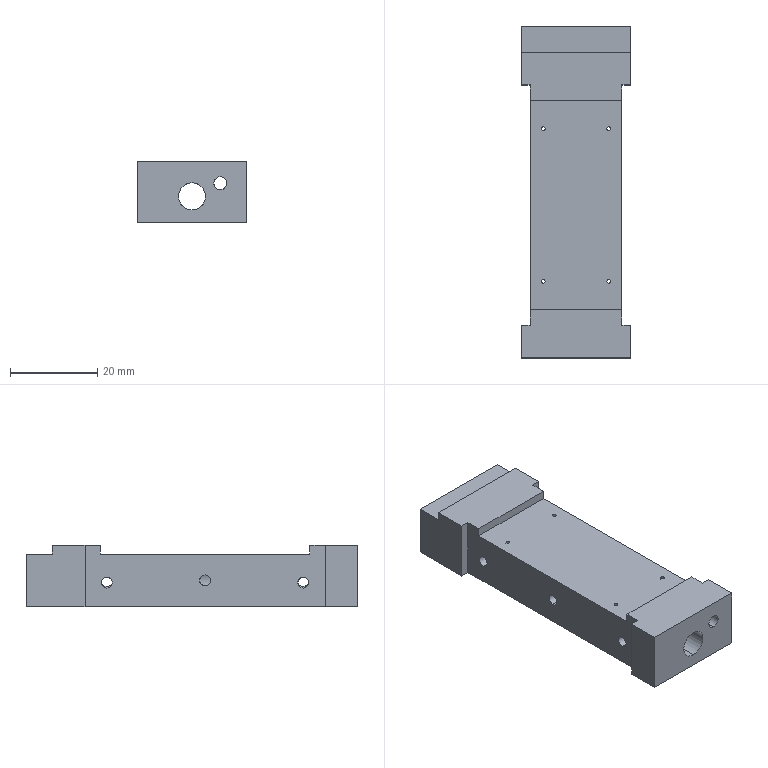Part | SolidWorks | features ICE 7, 3DProfileFeature 4, HoleWzd 4, Extrusion 1, MirrorPattern 1 | 1 solid | 70 faces | box 25 x 76 x 14 mm | volume 17689 mm3 | plane 30 | cylinder 26 | cone 14 | commonest cylinder face diameters 2.5 x20 3 x4 6.2 x2